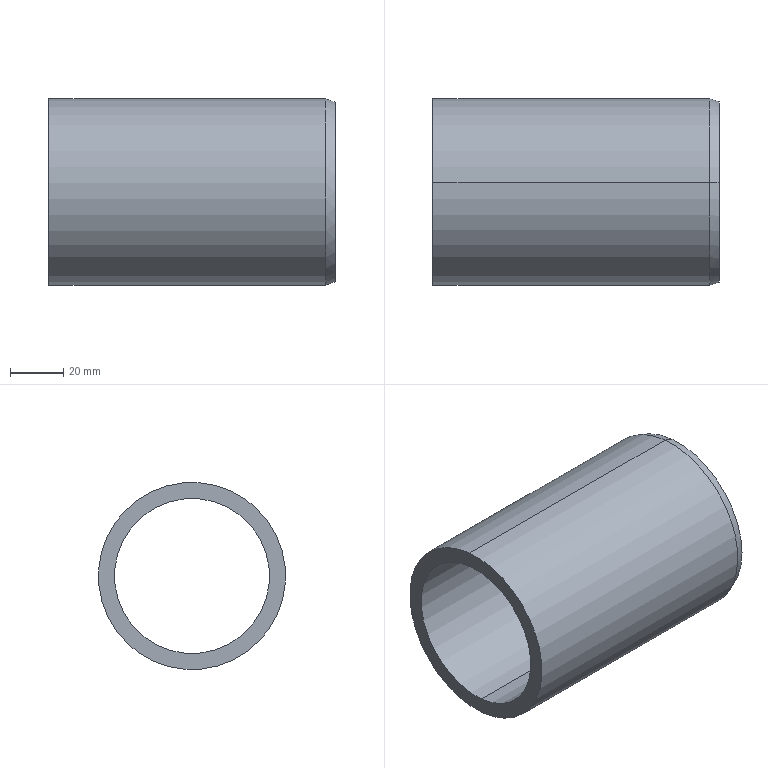Part | NX | features BREP 1 | 1 solid | 11 faces | box 107.08 x 70 x 70 mm | volume 125329 mm3 | cylinder 6 | plane 3 | cone 2 | commonest cylinder face diameters 58 x2 61 x2 70 x2
STEP:
#1=CARTESIAN_POINT('',(602.745,-3.343,-33.56));
#2=VERTEX_POINT('',#1);
#3=CARTESIAN_POINT('',(602.745,3.343,33.56));
#4=VERTEX_POINT('',#3);
#5=CARTESIAN_POINT('',(602.745,0.,0.));
#6=DIRECTION('',(1.,0.,0.));
#7=DIRECTION('',(0.,0.09911,0.9951));
#8=AXIS2_PLACEMENT_3D('',#5,#6,#7);
#9=CIRCLE('',#8,33.726);
#10=EDGE_CURVE('',#2,#4,#9,.T.);
#11=ORIENTED_EDGE('',*,*,#10,.F.);
#12=CARTESIAN_POINT('',(599.245,-3.469,-34.828));
#13=VERTEX_POINT('',#12);
#14=CARTESIAN_POINT('',(602.745,-3.343,-33.56));
#15=DIRECTION('',(-0.9397,-0.0339,-0.3403));
#16=VECTOR('',#15,1000.);
#17=LINE('',#14,#16);
#18=EDGE_CURVE('',#2,#13,#17,.T.);
#19=ORIENTED_EDGE('',*,*,#18,.T.);
#20=CARTESIAN_POINT('',(599.245,3.469,34.828));
#21=VERTEX_POINT('',#20);
#22=CARTESIAN_POINT('',(599.245,0.,0.));
#23=DIRECTION('',(-1.,0.,0.));
#24=DIRECTION('',(0.,0.09911,0.9951));
#25=AXIS2_PLACEMENT_3D('',#22,#23,#24);
#26=CIRCLE('',#25,35.);
#27=EDGE_CURVE('',#21,#13,#26,.T.);
#28=ORIENTED_EDGE('',*,*,#27,.F.);
#29=CARTESIAN_POINT('',(602.745,3.343,33.56));
#30=DIRECTION('',(-0.9397,0.0339,0.3403));
#31=VECTOR('',#30,1000.);
#32=LINE('',#29,#31);
#33=EDGE_CURVE('',#4,#21,#32,.T.);
#34=ORIENTED_EDGE('',*,*,#33,.F.);
#35=EDGE_LOOP('',(#11,#19,#28,#34));
#36=FACE_BOUND('',#35,.T.);
#37=CARTESIAN_POINT('',(602.745,0.,0.));
#38=DIRECTION('',(-1.,0.,0.));
#39=DIRECTION('',(0.,-0.09911,-0.9951));
#40=AXIS2_PLACEMENT_3D('',#37,#38,#39);
#41=CONICAL_SURFACE('',#40,33.726,0.3491);
#42=ADVANCED_FACE('',(#36),#41,.T.);
#43=CARTESIAN_POINT('',(590.745,3.023,30.35));
#44=VERTEX_POINT('',#43);
#45=CARTESIAN_POINT('',(590.745,-3.023,-30.35));
#46=VERTEX_POINT('',#45);
#47=CARTESIAN_POINT('',(590.745,0.,0.));
#48=DIRECTION('',(1.,0.,0.));
#49=DIRECTION('',(0.,-0.09911,-0.9951));
#50=AXIS2_PLACEMENT_3D('',#47,#48,#49);
#51=CIRCLE('',#50,30.5);
#52=EDGE_CURVE('',#44,#46,#51,.T.);
#53=ORIENTED_EDGE('',*,*,#52,.F.);
#54=CARTESIAN_POINT('',(602.745,3.023,30.35));
#55=VERTEX_POINT('',#54);
#56=CARTESIAN_POINT('',(602.745,3.023,30.35));
#57=DIRECTION('',(1.,0.,0.));
#58=VECTOR('',#57,1000.);
#59=LINE('',#56,#58);
#60=EDGE_CURVE('',#55,#44,#59,.F.);
#61=ORIENTED_EDGE('',*,*,#60,.F.);
#62=CARTESIAN_POINT('',(602.745,-3.023,-30.35));
#63=VERTEX_POINT('',#62);
#64=CARTESIAN_POINT('',(602.745,0.,0.));
#65=DIRECTION('',(1.,0.,0.));
#66=DIRECTION('',(0.,-0.09911,-0.9951));
#67=AXIS2_PLACEMENT_3D('',#64,#65,#66);
#68=CIRCLE('',#67,30.5);
#69=EDGE_CURVE('',#55,#63,#68,.T.);
#70=ORIENTED_EDGE('',*,*,#69,.T.);
#71=CARTESIAN_POINT('',(602.745,-3.023,-30.35));
#72=DIRECTION('',(1.,0.,0.));
#73=VECTOR('',#72,1000.);
#74=LINE('',#71,#73);
#75=EDGE_CURVE('',#63,#46,#74,.F.);
#76=ORIENTED_EDGE('',*,*,#75,.T.);
#77=EDGE_LOOP('',(#53,#61,#70,#76));
#78=FACE_BOUND('',#77,.T.);
#79=CARTESIAN_POINT('',(602.745,0.,0.));
#80=DIRECTION('',(1.,0.,0.));
#81=DIRECTION('',(0.,0.09911,0.9951));
#82=AXIS2_PLACEMENT_3D('',#79,#80,#81);
#83=CYLINDRICAL_SURFACE('',#82,30.5);
#84=ADVANCED_FACE('',(#78),#83,.F.);
#85=CARTESIAN_POINT('',(495.665,-2.874,-28.857));
#86=VERTEX_POINT('',#85);
#87=CARTESIAN_POINT('',(495.665,2.874,28.857));
#88=VERTEX_POINT('',#87);
#89=CARTESIAN_POINT('',(495.665,0.,0.));
#90=DIRECTION('',(-1.,0.,0.));
#91=DIRECTION('',(0.,0.,-1.));
#92=AXIS2_PLACEMENT_3D('',#89,#90,#91);
#93=CIRCLE('',#92,29.);
#94=EDGE_CURVE('',#86,#88,#93,.T.);
#95=ORIENTED_EDGE('',*,*,#94,.T.);
#96=CARTESIAN_POINT('',(590.745,2.874,28.857));
#97=VERTEX_POINT('',#96);
#98=CARTESIAN_POINT('',(602.745,2.874,28.857));
#99=DIRECTION('',(1.,0.,0.));
#100=VECTOR('',#99,1000.);
#101=LINE('',#98,#100);
#102=EDGE_CURVE('',#97,#88,#101,.F.);
#103=ORIENTED_EDGE('',*,*,#102,.F.);
#104=CARTESIAN_POINT('',(590.745,-2.874,-28.857));
#105=VERTEX_POINT('',#104);
#106=CARTESIAN_POINT('',(590.745,0.,0.));
#107=DIRECTION('',(1.,0.,0.));
#108=DIRECTION('',(0.,-0.09911,-0.9951));
#109=AXIS2_PLACEMENT_3D('',#106,#107,#108);
#110=CIRCLE('',#109,29.);
#111=EDGE_CURVE('',#97,#105,#110,.T.);
#112=ORIENTED_EDGE('',*,*,#111,.T.);
#113=CARTESIAN_POINT('',(602.745,-2.874,-28.857));
#114=DIRECTION('',(1.,0.,0.));
#115=VECTOR('',#114,1000.);
#116=LINE('',#113,#115);
#117=EDGE_CURVE('',#105,#86,#116,.F.);
#118=ORIENTED_EDGE('',*,*,#117,.T.);
#119=EDGE_LOOP('',(#95,#103,#112,#118));
#120=FACE_BOUND('',#119,.T.);
#121=CARTESIAN_POINT('',(602.745,0.,0.));
#122=DIRECTION('',(1.,0.,0.));
#123=DIRECTION('',(0.,0.09911,0.9951));
#124=AXIS2_PLACEMENT_3D('',#121,#122,#123);
#125=CYLINDRICAL_SURFACE('',#124,29.);
#126=ADVANCED_FACE('',(#120),#125,.F.);
#127=CARTESIAN_POINT('',(495.665,-3.469,-34.828));
#128=VERTEX_POINT('',#127);
#129=CARTESIAN_POINT('',(495.665,3.469,34.828));
#130=VERTEX_POINT('',#129);
#131=CARTESIAN_POINT('',(495.665,0.,0.));
#132=DIRECTION('',(1.,0.,0.));
#133=DIRECTION('',(0.,0.,-1.));
#134=AXIS2_PLACEMENT_3D('',#131,#132,#133);
#135=CIRCLE('',#134,35.);
#136=EDGE_CURVE('',#128,#130,#135,.T.);
#137=ORIENTED_EDGE('',*,*,#136,.T.);
#138=CARTESIAN_POINT('',(602.745,3.469,34.828));
#139=DIRECTION('',(1.,0.,0.));
#140=VECTOR('',#139,1000.);
#141=LINE('',#138,#140);
#142=EDGE_CURVE('',#21,#130,#141,.F.);
#143=ORIENTED_EDGE('',*,*,#142,.F.);
#144=ORIENTED_EDGE('',*,*,#27,.T.);
#145=CARTESIAN_POINT('',(602.745,-3.469,-34.828));
#146=DIRECTION('',(1.,0.,0.));
#147=VECTOR('',#146,1000.);
#148=LINE('',#145,#147);
#149=EDGE_CURVE('',#13,#128,#148,.F.);
#150=ORIENTED_EDGE('',*,*,#149,.T.);
#151=EDGE_LOOP('',(#137,#143,#144,#150));
#152=FACE_BOUND('',#151,.T.);
#153=CARTESIAN_POINT('',(602.745,0.,0.));
#154=DIRECTION('',(1.,0.,0.));
#155=DIRECTION('',(0.,0.09911,0.9951));
#156=AXIS2_PLACEMENT_3D('',#153,#154,#155);
#157=CYLINDRICAL_SURFACE('',#156,35.);
#158=ADVANCED_FACE('',(#152),#157,.T.);
#159=ORIENTED_EDGE('',*,*,#142,.T.);
#160=CARTESIAN_POINT('',(495.665,0.,0.));
#161=DIRECTION('',(1.,0.,0.));
#162=DIRECTION('',(0.,0.,-1.));
#163=AXIS2_PLACEMENT_3D('',#160,#161,#162);
#164=CIRCLE('',#163,35.);
#165=EDGE_CURVE('',#130,#128,#164,.T.);
#166=ORIENTED_EDGE('',*,*,#165,.T.);
#167=ORIENTED_EDGE('',*,*,#149,.F.);
#168=CARTESIAN_POINT('',(599.245,0.,0.));
#169=DIRECTION('',(-1.,0.,0.));
#170=DIRECTION('',(0.,0.09911,0.9951));
#171=AXIS2_PLACEMENT_3D('',#168,#169,#170);
#172=CIRCLE('',#171,35.);
#173=EDGE_CURVE('',#13,#21,#172,.T.);
#174=ORIENTED_EDGE('',*,*,#173,.T.);
#175=EDGE_LOOP('',(#159,#166,#167,#174));
#176=FACE_BOUND('',#175,.T.);
#177=CARTESIAN_POINT('',(602.745,0.,0.));
#178=DIRECTION('',(1.,0.,0.));
#179=DIRECTION('',(0.,0.09911,0.9951));
#180=AXIS2_PLACEMENT_3D('',#177,#178,#179);
#181=CYLINDRICAL_SURFACE('',#180,35.);
#182=ADVANCED_FACE('',(#176),#181,.T.);
#183=CARTESIAN_POINT('',(602.745,0.,0.));
#184=DIRECTION('',(1.,0.,0.));
#185=DIRECTION('',(0.,0.09911,0.9951));
#186=AXIS2_PLACEMENT_3D('',#183,#184,#185);
#187=CIRCLE('',#186,33.726);
#188=EDGE_CURVE('',#4,#2,#187,.T.);
#189=ORIENTED_EDGE('',*,*,#188,.T.);
#190=ORIENTED_EDGE('',*,*,#10,.T.);
#191=EDGE_LOOP('',(#189,#190));
#192=FACE_BOUND('',#191,.T.);
#193=CARTESIAN_POINT('',(602.745,0.,0.));
#194=DIRECTION('',(1.,0.,0.));
#195=DIRECTION('',(0.,-0.09911,-0.9951));
#196=AXIS2_PLACEMENT_3D('',#193,#194,#195);
#197=CIRCLE('',#196,30.5);
#198=EDGE_CURVE('',#63,#55,#197,.T.);
#199=ORIENTED_EDGE('',*,*,#198,.F.);
#200=ORIENTED_EDGE('',*,*,#69,.F.);
#201=EDGE_LOOP('',(#199,#200));
#202=FACE_BOUND('',#201,.T.);
#203=CARTESIAN_POINT('',(602.745,34.828,-3.469));
#204=DIRECTION('',(-1.,0.,0.));
#205=DIRECTION('',(0.,-0.09911,-0.9951));
#206=AXIS2_PLACEMENT_3D('',#203,#204,#205);
#207=PLANE('',#206);
#208=ADVANCED_FACE('',(#192,#202),#207,.F.);
#209=ORIENTED_EDGE('',*,*,#102,.T.);
#210=CARTESIAN_POINT('',(495.665,0.,0.));
#211=DIRECTION('',(-1.,0.,0.));
#212=DIRECTION('',(0.,0.,-1.));
#213=AXIS2_PLACEMENT_3D('',#210,#211,#212);
#214=CIRCLE('',#213,29.);
#215=EDGE_CURVE('',#88,#86,#214,.T.);
#216=ORIENTED_EDGE('',*,*,#215,.T.);
#217=ORIENTED_EDGE('',*,*,#117,.F.);
#218=CARTESIAN_POINT('',(590.745,0.,0.));
#219=DIRECTION('',(1.,0.,0.));
#220=DIRECTION('',(0.,-0.09911,-0.9951));
#221=AXIS2_PLACEMENT_3D('',#218,#219,#220);
#222=CIRCLE('',#221,29.);
#223=EDGE_CURVE('',#105,#97,#222,.T.);
#224=ORIENTED_EDGE('',*,*,#223,.T.);
#225=EDGE_LOOP('',(#209,#216,#217,#224));
#226=FACE_BOUND('',#225,.T.);
#227=CARTESIAN_POINT('',(602.745,0.,0.));
#228=DIRECTION('',(1.,0.,0.));
#229=DIRECTION('',(0.,0.09911,0.9951));
#230=AXIS2_PLACEMENT_3D('',#227,#228,#229);
#231=CYLINDRICAL_SURFACE('',#230,29.);
#232=ADVANCED_FACE('',(#226),#231,.F.);
#233=ORIENTED_EDGE('',*,*,#223,.F.);
#234=ORIENTED_EDGE('',*,*,#111,.F.);
#235=EDGE_LOOP('',(#233,#234));
#236=FACE_BOUND('',#235,.T.);
#237=CARTESIAN_POINT('',(590.745,0.,0.));
#238=DIRECTION('',(1.,0.,0.));
#239=DIRECTION('',(0.,-0.09911,-0.9951));
#240=AXIS2_PLACEMENT_3D('',#237,#238,#239);
#241=CIRCLE('',#240,30.5);
#242=EDGE_CURVE('',#46,#44,#241,.T.);
#243=ORIENTED_EDGE('',*,*,#242,.T.);
#244=ORIENTED_EDGE('',*,*,#52,.T.);
#245=EDGE_LOOP('',(#243,#244));
#246=FACE_BOUND('',#245,.T.);
#247=CARTESIAN_POINT('',(590.745,28.857,-2.874));
#248=DIRECTION('',(-1.,0.,0.));
#249=DIRECTION('',(0.,-0.09911,-0.9951));
#250=AXIS2_PLACEMENT_3D('',#247,#248,#249);
#251=PLANE('',#250);
#252=ADVANCED_FACE('',(#236,#246),#251,.F.);
#253=ORIENTED_EDGE('',*,*,#60,.T.);
#254=ORIENTED_EDGE('',*,*,#242,.F.);
#255=ORIENTED_EDGE('',*,*,#75,.F.);
#256=ORIENTED_EDGE('',*,*,#198,.T.);
#257=EDGE_LOOP('',(#253,#254,#255,#256));
#258=FACE_BOUND('',#257,.T.);
#259=CARTESIAN_POINT('',(602.745,0.,0.));
#260=DIRECTION('',(1.,0.,0.));
#261=DIRECTION('',(0.,0.09911,0.9951));
#262=AXIS2_PLACEMENT_3D('',#259,#260,#261);
#263=CYLINDRICAL_SURFACE('',#262,30.5);
#264=ADVANCED_FACE('',(#258),#263,.F.);
#265=ORIENTED_EDGE('',*,*,#18,.F.);
#266=ORIENTED_EDGE('',*,*,#188,.F.);
#267=ORIENTED_EDGE('',*,*,#33,.T.);
#268=ORIENTED_EDGE('',*,*,#173,.F.);
#269=EDGE_LOOP('',(#265,#266,#267,#268));
#270=FACE_BOUND('',#269,.T.);
#271=CARTESIAN_POINT('',(602.745,0.,0.));
#272=DIRECTION('',(-1.,0.,0.));
#273=DIRECTION('',(0.,-0.09911,-0.9951));
#274=AXIS2_PLACEMENT_3D('',#271,#272,#273);
#275=CONICAL_SURFACE('',#274,33.726,0.3491);
#276=ADVANCED_FACE('',(#270),#275,.T.);
#277=ORIENTED_EDGE('',*,*,#94,.F.);
#278=ORIENTED_EDGE('',*,*,#215,.F.);
#279=EDGE_LOOP('',(#277,#278));
#280=FACE_BOUND('',#279,.T.);
#281=ORIENTED_EDGE('',*,*,#136,.F.);
#282=ORIENTED_EDGE('',*,*,#165,.F.);
#283=EDGE_LOOP('',(#281,#282));
#284=FACE_BOUND('',#283,.T.);
#285=CARTESIAN_POINT('',(495.665,-40.903,-44.627));
#286=DIRECTION('',(1.,0.,0.));
#287=DIRECTION('',(0.,0.,1.));
#288=AXIS2_PLACEMENT_3D('',#285,#286,#287);
#289=PLANE('',#288);
#290=ADVANCED_FACE('',(#280,#284),#289,.F.);
#291=CLOSED_SHELL('',(#42,#84,#126,#158,#182,#208,#232,#252,#264,#276,#290));
#292=MANIFOLD_SOLID_BREP('',#291);
#293=(LENGTH_UNIT()NAMED_UNIT(*)SI_UNIT(.MILLI.,.METRE.));
#294=UNCERTAINTY_MEASURE_WITH_UNIT(LENGTH_MEASURE(0.00001),#293,'','');
#295=(NAMED_UNIT(*)PLANE_ANGLE_UNIT()SI_UNIT($,.RADIAN.));
#296=(NAMED_UNIT(*)SI_UNIT($,.STERADIAN.)SOLID_ANGLE_UNIT());
#297=(GEOMETRIC_REPRESENTATION_CONTEXT(3)GLOBAL_UNCERTAINTY_ASSIGNED_CONTEXT((#294))GLOBAL_UNIT_ASSIGNED_CONTEXT((#293,#295,#296))REPRESENTATION_CONTEXT('',''));
#298=ADVANCED_BREP_SHAPE_REPRESENTATION('',(#292),#297);